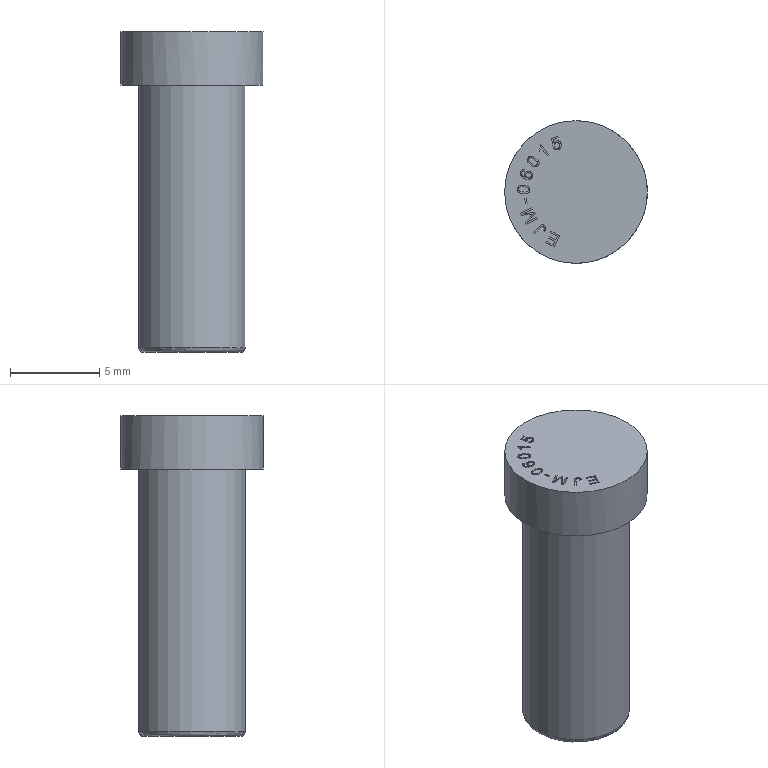Part | NX | features solid 2 | 1 solid | 85 faces | box 8 x 8 x 18 mm | volume 574.318 mm3 | plane 57 | spline 25 | cylinder 2 | torus 1 | commonest cylinder face diameters 6 x1 8 x1